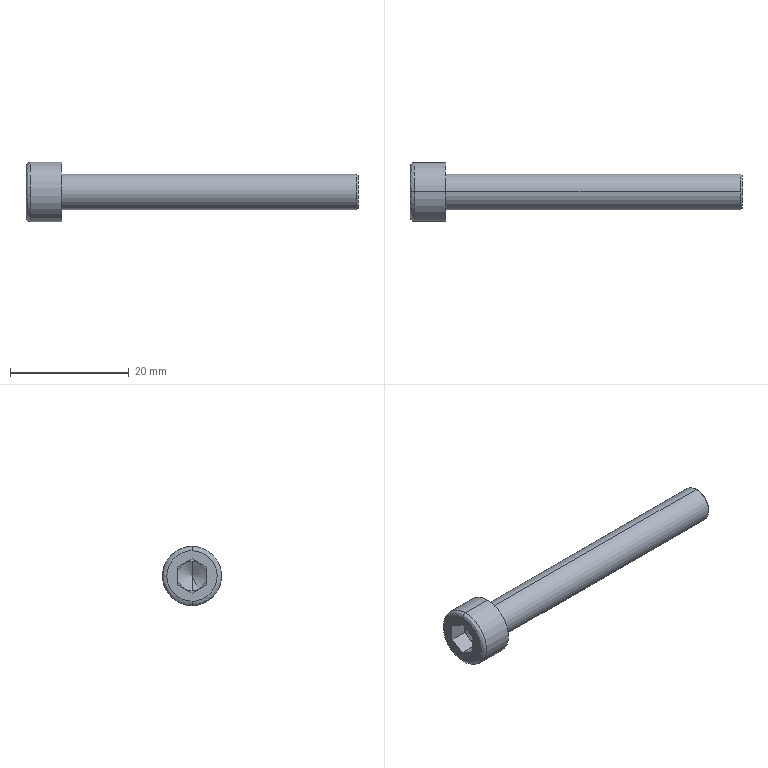Part | STEP file | hexagon socket head cap screws gb_GB_FASTENER_SCREWS_HSHCS M6X50-N | 1 solid | 25 faces | box 56 x 10 x 10 mm | volume 1806 mm3 | plane 15 | cylinder 4 | cone 4 | spline 2 | commonest cylinder face diameters 6 x2 10 x2
STEP:
#1=CARTESIAN_POINT('',(0.75,0.,5.));
#2=VERTEX_POINT('',#1);
#3=CARTESIAN_POINT('',(0.75,0.,-5.));
#4=VERTEX_POINT('',#3);
#5=CARTESIAN_POINT('',(0.75,0.,0.));
#6=DIRECTION('',(1.,0.,0.));
#7=DIRECTION('',(0.,0.,1.));
#8=AXIS2_PLACEMENT_3D('',#5,#6,#7);
#9=CIRCLE('',#8,5.);
#10=EDGE_CURVE('',#2,#4,#9,.T.);
#11=ORIENTED_EDGE('',*,*,#10,.F.);
#12=CARTESIAN_POINT('',(0.,0.,4.25));
#13=VERTEX_POINT('',#12);
#14=CARTESIAN_POINT('',(0.75,0.,4.25));
#15=DIRECTION('',(0.,-1.,0.));
#16=DIRECTION('',(0.,0.,1.));
#17=AXIS2_PLACEMENT_3D('',#14,#15,#16);
#18=CIRCLE('',#17,0.75);
#19=EDGE_CURVE('',#2,#13,#18,.T.);
#20=ORIENTED_EDGE('',*,*,#19,.T.);
#21=CARTESIAN_POINT('',(0.,0.,-4.25));
#22=VERTEX_POINT('',#21);
#23=CARTESIAN_POINT('',(0.,0.,4.25));
#24=CARTESIAN_POINT('',(0.,-8.5,4.25));
#25=CARTESIAN_POINT('',(0.,-8.5,-4.25));
#26=CARTESIAN_POINT('',(0.,0.,-4.25));
#27=(BOUNDED_CURVE()B_SPLINE_CURVE(3,(#23,#24,#25,#26),.UNSPECIFIED.,.F.,.F.)B_SPLINE_CURVE_WITH_KNOTS((4,4),(0.,1.),.UNSPECIFIED.)CURVE()GEOMETRIC_REPRESENTATION_ITEM()RATIONAL_B_SPLINE_CURVE((1.,0.3333,0.3333,1.))REPRESENTATION_ITEM(''));
#28=EDGE_CURVE('',#13,#22,#27,.T.);
#29=ORIENTED_EDGE('',*,*,#28,.T.);
#30=CARTESIAN_POINT('',(0.75,0.,-4.25));
#31=DIRECTION('',(0.,1.,0.));
#32=DIRECTION('',(0.,0.,-1.));
#33=AXIS2_PLACEMENT_3D('',#30,#31,#32);
#34=CIRCLE('',#33,0.75);
#35=EDGE_CURVE('',#4,#22,#34,.T.);
#36=ORIENTED_EDGE('',*,*,#35,.F.);
#37=EDGE_LOOP('',(#11,#20,#29,#36));
#38=FACE_OUTER_BOUND('',#37,.T.);
#39=CARTESIAN_POINT('',(0.75,0.,5.));
#40=CARTESIAN_POINT('',(0.75,-10.,5.));
#41=CARTESIAN_POINT('',(0.75,-10.,-5.));
#42=CARTESIAN_POINT('',(0.75,0.,-5.));
#43=CARTESIAN_POINT('',(0.3107,0.,5.));
#44=CARTESIAN_POINT('',(0.3107,-10.,5.));
#45=CARTESIAN_POINT('',(0.3107,-10.,-5.));
#46=CARTESIAN_POINT('',(0.3107,0.,-5.));
#47=CARTESIAN_POINT('',(0.,0.,4.689));
#48=CARTESIAN_POINT('',(0.,-9.379,4.689));
#49=CARTESIAN_POINT('',(0.,-9.379,-4.689));
#50=CARTESIAN_POINT('',(0.,0.,-4.689));
#51=CARTESIAN_POINT('',(0.,0.,4.25));
#52=CARTESIAN_POINT('',(0.,-8.5,4.25));
#53=CARTESIAN_POINT('',(0.,-8.5,-4.25));
#54=CARTESIAN_POINT('',(0.,0.,-4.25));
#55=(BOUNDED_SURFACE()B_SPLINE_SURFACE(3,3,((#39,#40,#41,#42),(#43,#44,#45,#46),(#47,#48,#49,#50),(#51,#52,#53,#54)),.UNSPECIFIED.,.F.,.F.,.F.)B_SPLINE_SURFACE_WITH_KNOTS((4,4),(4,4),(0.,1.),(0.,1.),.UNSPECIFIED.)GEOMETRIC_REPRESENTATION_ITEM()RATIONAL_B_SPLINE_SURFACE(((1.,0.3333,0.3333,1.),(0.8047,0.2682,0.2682,0.8047),(0.8047,0.2682,0.2682,0.8047),(1.,0.3333,0.3333,1.)))REPRESENTATION_ITEM('')SURFACE());
#56=ADVANCED_FACE('',(#38),#55,.T.);
#57=CARTESIAN_POINT('',(55.75,0.,3.));
#58=VERTEX_POINT('',#57);
#59=CARTESIAN_POINT('',(55.75,0.,-3.));
#60=VERTEX_POINT('',#59);
#61=CARTESIAN_POINT('',(55.75,0.,0.));
#62=DIRECTION('',(-1.,0.,0.));
#63=DIRECTION('',(0.,0.,1.));
#64=AXIS2_PLACEMENT_3D('',#61,#62,#63);
#65=CIRCLE('',#64,3.);
#66=EDGE_CURVE('',#58,#60,#65,.T.);
#67=ORIENTED_EDGE('',*,*,#66,.T.);
#68=CARTESIAN_POINT('',(6.,0.,-3.));
#69=VERTEX_POINT('',#68);
#70=CARTESIAN_POINT('',(56.,0.,-3.));
#71=DIRECTION('',(-1.,0.,0.));
#72=VECTOR('',#71,1000.);
#73=LINE('',#70,#72);
#74=EDGE_CURVE('',#60,#69,#73,.T.);
#75=ORIENTED_EDGE('',*,*,#74,.T.);
#76=CARTESIAN_POINT('',(6.,0.,3.));
#77=VERTEX_POINT('',#76);
#78=CARTESIAN_POINT('',(6.,0.,0.));
#79=DIRECTION('',(1.,0.,0.));
#80=DIRECTION('',(0.,0.,1.));
#81=AXIS2_PLACEMENT_3D('',#78,#79,#80);
#82=CIRCLE('',#81,3.);
#83=EDGE_CURVE('',#69,#77,#82,.T.);
#84=ORIENTED_EDGE('',*,*,#83,.T.);
#85=CARTESIAN_POINT('',(56.,0.,3.));
#86=DIRECTION('',(-1.,0.,0.));
#87=VECTOR('',#86,1000.);
#88=LINE('',#85,#87);
#89=EDGE_CURVE('',#58,#77,#88,.T.);
#90=ORIENTED_EDGE('',*,*,#89,.F.);
#91=EDGE_LOOP('',(#67,#75,#84,#90));
#92=FACE_OUTER_BOUND('',#91,.T.);
#93=CARTESIAN_POINT('',(56.,0.,0.));
#94=DIRECTION('',(-1.,0.,0.));
#95=DIRECTION('',(0.,0.,1.));
#96=AXIS2_PLACEMENT_3D('',#93,#94,#95);
#97=CYLINDRICAL_SURFACE('',#96,3.);
#98=ADVANCED_FACE('',(#92),#97,.T.);
#99=CARTESIAN_POINT('',(56.,0.,2.75));
#100=VERTEX_POINT('',#99);
#101=CARTESIAN_POINT('',(56.,0.,-2.75));
#102=VERTEX_POINT('',#101);
#103=CARTESIAN_POINT('',(56.,0.,0.));
#104=DIRECTION('',(-1.,0.,0.));
#105=DIRECTION('',(0.,0.,1.));
#106=AXIS2_PLACEMENT_3D('',#103,#104,#105);
#107=CIRCLE('',#106,2.75);
#108=EDGE_CURVE('',#100,#102,#107,.T.);
#109=ORIENTED_EDGE('',*,*,#108,.T.);
#110=CARTESIAN_POINT('',(55.75,0.,-3.));
#111=DIRECTION('',(-0.7071,0.,-0.7071));
#112=VECTOR('',#111,1000.);
#113=LINE('',#110,#112);
#114=EDGE_CURVE('',#102,#60,#113,.T.);
#115=ORIENTED_EDGE('',*,*,#114,.T.);
#116=ORIENTED_EDGE('',*,*,#66,.F.);
#117=CARTESIAN_POINT('',(55.75,0.,3.));
#118=DIRECTION('',(-0.7071,0.,0.7071));
#119=VECTOR('',#118,1000.);
#120=LINE('',#117,#119);
#121=EDGE_CURVE('',#100,#58,#120,.T.);
#122=ORIENTED_EDGE('',*,*,#121,.F.);
#123=EDGE_LOOP('',(#109,#115,#116,#122));
#124=FACE_OUTER_BOUND('',#123,.T.);
#125=CARTESIAN_POINT('',(55.75,0.,0.));
#126=DIRECTION('',(-1.,0.,0.));
#127=DIRECTION('',(0.,0.,1.));
#128=AXIS2_PLACEMENT_3D('',#125,#126,#127);
#129=CONICAL_SURFACE('',#128,3.,0.7854);
#130=ADVANCED_FACE('',(#124),#129,.T.);
#131=CARTESIAN_POINT('',(6.,0.,-5.));
#132=VERTEX_POINT('',#131);
#133=CARTESIAN_POINT('',(6.,0.,5.));
#134=VERTEX_POINT('',#133);
#135=CARTESIAN_POINT('',(6.,0.,0.));
#136=DIRECTION('',(1.,0.,0.));
#137=DIRECTION('',(0.,0.,1.));
#138=AXIS2_PLACEMENT_3D('',#135,#136,#137);
#139=CIRCLE('',#138,5.);
#140=EDGE_CURVE('',#132,#134,#139,.T.);
#141=ORIENTED_EDGE('',*,*,#140,.F.);
#142=CARTESIAN_POINT('',(6.,0.,-5.));
#143=DIRECTION('',(-1.,0.,0.));
#144=VECTOR('',#143,1000.);
#145=LINE('',#142,#144);
#146=EDGE_CURVE('',#132,#4,#145,.T.);
#147=ORIENTED_EDGE('',*,*,#146,.T.);
#148=CARTESIAN_POINT('',(0.75,0.,0.));
#149=DIRECTION('',(1.,0.,0.));
#150=DIRECTION('',(0.,0.,1.));
#151=AXIS2_PLACEMENT_3D('',#148,#149,#150);
#152=CIRCLE('',#151,5.);
#153=EDGE_CURVE('',#4,#2,#152,.T.);
#154=ORIENTED_EDGE('',*,*,#153,.T.);
#155=CARTESIAN_POINT('',(6.,0.,5.));
#156=DIRECTION('',(-1.,0.,0.));
#157=VECTOR('',#156,1000.);
#158=LINE('',#155,#157);
#159=EDGE_CURVE('',#134,#2,#158,.T.);
#160=ORIENTED_EDGE('',*,*,#159,.F.);
#161=EDGE_LOOP('',(#141,#147,#154,#160));
#162=FACE_OUTER_BOUND('',#161,.T.);
#163=CARTESIAN_POINT('',(6.,0.,0.));
#164=DIRECTION('',(-1.,0.,0.));
#165=DIRECTION('',(0.,0.,1.));
#166=AXIS2_PLACEMENT_3D('',#163,#164,#165);
#167=CYLINDRICAL_SURFACE('',#166,5.);
#168=ADVANCED_FACE('',(#162),#167,.T.);
#169=CARTESIAN_POINT('',(4.443,0.,0.));
#170=VERTEX_POINT('',#169);
#171=CARTESIAN_POINT('',(3.,0.,2.5));
#172=VERTEX_POINT('',#171);
#173=CARTESIAN_POINT('',(3.,0.,2.5));
#174=DIRECTION('',(-0.5,0.,0.866));
#175=VECTOR('',#174,1000.);
#176=LINE('',#173,#175);
#177=EDGE_CURVE('',#170,#172,#176,.T.);
#178=ORIENTED_EDGE('',*,*,#177,.F.);
#179=CARTESIAN_POINT('',(3.,0.,-2.5));
#180=VERTEX_POINT('',#179);
#181=CARTESIAN_POINT('',(3.,0.,-2.5));
#182=DIRECTION('',(-0.5,0.,-0.866));
#183=VECTOR('',#182,1000.);
#184=LINE('',#181,#183);
#185=EDGE_CURVE('',#170,#180,#184,.T.);
#186=ORIENTED_EDGE('',*,*,#185,.T.);
#187=CARTESIAN_POINT('',(3.,-1.25,-2.165));
#188=VERTEX_POINT('',#187);
#189=CARTESIAN_POINT('',(3.,0.,0.));
#190=DIRECTION('',(1.,0.,0.));
#191=DIRECTION('',(0.,0.,1.));
#192=AXIS2_PLACEMENT_3D('',#189,#190,#191);
#193=CIRCLE('',#192,2.5);
#194=EDGE_CURVE('',#188,#180,#193,.T.);
#195=ORIENTED_EDGE('',*,*,#194,.F.);
#196=CARTESIAN_POINT('',(3.,-2.5,0.));
#197=VERTEX_POINT('',#196);
#198=CARTESIAN_POINT('',(3.,0.,0.));
#199=DIRECTION('',(1.,0.,0.));
#200=DIRECTION('',(0.,0.,1.));
#201=AXIS2_PLACEMENT_3D('',#198,#199,#200);
#202=CIRCLE('',#201,2.5);
#203=EDGE_CURVE('',#197,#188,#202,.T.);
#204=ORIENTED_EDGE('',*,*,#203,.F.);
#205=CARTESIAN_POINT('',(3.,-1.25,2.165));
#206=VERTEX_POINT('',#205);
#207=CARTESIAN_POINT('',(3.,0.,0.));
#208=DIRECTION('',(-1.,0.,0.));
#209=DIRECTION('',(0.,0.,1.));
#210=AXIS2_PLACEMENT_3D('',#207,#208,#209);
#211=CIRCLE('',#210,2.5);
#212=EDGE_CURVE('',#197,#206,#211,.T.);
#213=ORIENTED_EDGE('',*,*,#212,.T.);
#214=CARTESIAN_POINT('',(3.,0.,0.));
#215=DIRECTION('',(1.,0.,0.));
#216=DIRECTION('',(0.,0.,1.));
#217=AXIS2_PLACEMENT_3D('',#214,#215,#216);
#218=CIRCLE('',#217,2.5);
#219=EDGE_CURVE('',#172,#206,#218,.T.);
#220=ORIENTED_EDGE('',*,*,#219,.F.);
#221=EDGE_LOOP('',(#178,#186,#195,#204,#213,#220));
#222=FACE_OUTER_BOUND('',#221,.T.);
#223=CARTESIAN_POINT('',(3.,0.,0.));
#224=DIRECTION('',(-1.,0.,0.));
#225=DIRECTION('',(0.,0.,1.));
#226=AXIS2_PLACEMENT_3D('',#223,#224,#225);
#227=CONICAL_SURFACE('',#226,2.5,1.047);
#228=ADVANCED_FACE('',(#222),#227,.F.);
#229=ORIENTED_EDGE('',*,*,#74,.F.);
#230=CARTESIAN_POINT('',(55.75,0.,0.));
#231=DIRECTION('',(-1.,0.,0.));
#232=DIRECTION('',(0.,0.,1.));
#233=AXIS2_PLACEMENT_3D('',#230,#231,#232);
#234=CIRCLE('',#233,3.);
#235=EDGE_CURVE('',#60,#58,#234,.T.);
#236=ORIENTED_EDGE('',*,*,#235,.T.);
#237=ORIENTED_EDGE('',*,*,#89,.T.);
#238=CARTESIAN_POINT('',(6.,0.,0.));
#239=DIRECTION('',(1.,0.,0.));
#240=DIRECTION('',(0.,0.,1.));
#241=AXIS2_PLACEMENT_3D('',#238,#239,#240);
#242=CIRCLE('',#241,3.);
#243=EDGE_CURVE('',#77,#69,#242,.T.);
#244=ORIENTED_EDGE('',*,*,#243,.T.);
#245=EDGE_LOOP('',(#229,#236,#237,#244));
#246=FACE_OUTER_BOUND('',#245,.T.);
#247=CARTESIAN_POINT('',(56.,0.,0.));
#248=DIRECTION('',(-1.,0.,0.));
#249=DIRECTION('',(0.,0.,1.));
#250=AXIS2_PLACEMENT_3D('',#247,#248,#249);
#251=CYLINDRICAL_SURFACE('',#250,3.);
#252=ADVANCED_FACE('',(#246),#251,.T.);
#253=ORIENTED_EDGE('',*,*,#243,.F.);
#254=ORIENTED_EDGE('',*,*,#83,.F.);
#255=EDGE_LOOP('',(#253,#254));
#256=FACE_BOUND('',#255,.T.);
#257=CARTESIAN_POINT('',(6.,0.,0.));
#258=DIRECTION('',(1.,0.,0.));
#259=DIRECTION('',(0.,0.,1.));
#260=AXIS2_PLACEMENT_3D('',#257,#258,#259);
#261=CIRCLE('',#260,5.);
#262=EDGE_CURVE('',#134,#132,#261,.T.);
#263=ORIENTED_EDGE('',*,*,#262,.T.);
#264=ORIENTED_EDGE('',*,*,#140,.T.);
#265=EDGE_LOOP('',(#263,#264));
#266=FACE_OUTER_BOUND('',#265,.T.);
#267=CARTESIAN_POINT('',(6.,0.,0.));
#268=DIRECTION('',(1.,0.,0.));
#269=DIRECTION('',(0.,0.,-1.));
#270=AXIS2_PLACEMENT_3D('',#267,#268,#269);
#271=PLANE('',#270);
#272=ADVANCED_FACE('',(#256,#266),#271,.T.);
#273=ORIENTED_EDGE('',*,*,#114,.F.);
#274=CARTESIAN_POINT('',(56.,0.,0.));
#275=DIRECTION('',(-1.,0.,0.));
#276=DIRECTION('',(0.,0.,1.));
#277=AXIS2_PLACEMENT_3D('',#274,#275,#276);
#278=CIRCLE('',#277,2.75);
#279=EDGE_CURVE('',#102,#100,#278,.T.);
#280=ORIENTED_EDGE('',*,*,#279,.T.);
#281=ORIENTED_EDGE('',*,*,#121,.T.);
#282=ORIENTED_EDGE('',*,*,#235,.F.);
#283=EDGE_LOOP('',(#273,#280,#281,#282));
#284=FACE_OUTER_BOUND('',#283,.T.);
#285=CARTESIAN_POINT('',(55.75,0.,0.));
#286=DIRECTION('',(-1.,0.,0.));
#287=DIRECTION('',(0.,0.,1.));
#288=AXIS2_PLACEMENT_3D('',#285,#286,#287);
#289=CONICAL_SURFACE('',#288,3.,0.7854);
#290=ADVANCED_FACE('',(#284),#289,.T.);
#291=ORIENTED_EDGE('',*,*,#146,.F.);
#292=ORIENTED_EDGE('',*,*,#262,.F.);
#293=ORIENTED_EDGE('',*,*,#159,.T.);
#294=ORIENTED_EDGE('',*,*,#10,.T.);
#295=EDGE_LOOP('',(#291,#292,#293,#294));
#296=FACE_OUTER_BOUND('',#295,.T.);
#297=CARTESIAN_POINT('',(6.,0.,0.));
#298=DIRECTION('',(-1.,0.,0.));
#299=DIRECTION('',(0.,0.,1.));
#300=AXIS2_PLACEMENT_3D('',#297,#298,#299);
#301=CYLINDRICAL_SURFACE('',#300,5.);
#302=ADVANCED_FACE('',(#296),#301,.T.);
#303=ORIENTED_EDGE('',*,*,#108,.F.);
#304=ORIENTED_EDGE('',*,*,#279,.F.);
#305=EDGE_LOOP('',(#303,#304));
#306=FACE_OUTER_BOUND('',#305,.T.);
#307=CARTESIAN_POINT('',(56.,0.,0.));
#308=DIRECTION('',(1.,0.,0.));
#309=DIRECTION('',(0.,0.,-1.));
#310=AXIS2_PLACEMENT_3D('',#307,#308,#309);
#311=PLANE('',#310);
#312=ADVANCED_FACE('',(#306),#311,.T.);
#313=ORIENTED_EDGE('',*,*,#19,.F.);
#314=ORIENTED_EDGE('',*,*,#153,.F.);
#315=ORIENTED_EDGE('',*,*,#35,.T.);
#316=CARTESIAN_POINT('',(0.,0.,-4.25));
#317=CARTESIAN_POINT('',(0.,8.5,-4.25));
#318=CARTESIAN_POINT('',(0.,8.5,4.25));
#319=CARTESIAN_POINT('',(0.,0.,4.25));
#320=(BOUNDED_CURVE()B_SPLINE_CURVE(3,(#316,#317,#318,#319),.UNSPECIFIED.,.F.,.F.)B_SPLINE_CURVE_WITH_KNOTS((4,4),(0.,1.),.UNSPECIFIED.)CURVE()GEOMETRIC_REPRESENTATION_ITEM()RATIONAL_B_SPLINE_CURVE((1.,0.3333,0.3333,1.))REPRESENTATION_ITEM(''));
#321=EDGE_CURVE('',#22,#13,#320,.T.);
#322=ORIENTED_EDGE('',*,*,#321,.T.);
#323=EDGE_LOOP('',(#313,#314,#315,#322));
#324=FACE_OUTER_BOUND('',#323,.T.);
#325=CARTESIAN_POINT('',(0.75,0.,-5.));
#326=CARTESIAN_POINT('',(0.75,10.,-5.));
#327=CARTESIAN_POINT('',(0.75,10.,5.));
#328=CARTESIAN_POINT('',(0.75,0.,5.));
#329=CARTESIAN_POINT('',(0.3107,0.,-5.));
#330=CARTESIAN_POINT('',(0.3107,10.,-5.));
#331=CARTESIAN_POINT('',(0.3107,10.,5.));
#332=CARTESIAN_POINT('',(0.3107,0.,5.));
#333=CARTESIAN_POINT('',(0.,0.,-4.689));
#334=CARTESIAN_POINT('',(0.,9.379,-4.689));
#335=CARTESIAN_POINT('',(0.,9.379,4.689));
#336=CARTESIAN_POINT('',(0.,0.,4.689));
#337=CARTESIAN_POINT('',(0.,0.,-4.25));
#338=CARTESIAN_POINT('',(0.,8.5,-4.25));
#339=CARTESIAN_POINT('',(0.,8.5,4.25));
#340=CARTESIAN_POINT('',(0.,0.,4.25));
#341=(BOUNDED_SURFACE()B_SPLINE_SURFACE(3,3,((#325,#326,#327,#328),(#329,#330,#331,#332),(#333,#334,#335,#336),(#337,#338,#339,#340)),.UNSPECIFIED.,.F.,.F.,.F.)B_SPLINE_SURFACE_WITH_KNOTS((4,4),(4,4),(0.,1.),(0.,1.),.UNSPECIFIED.)GEOMETRIC_REPRESENTATION_ITEM()RATIONAL_B_SPLINE_SURFACE(((1.,0.3333,0.3333,1.),(0.8047,0.2682,0.2682,0.8047),(0.8047,0.2682,0.2682,0.8047),(1.,0.3333,0.3333,1.)))REPRESENTATION_ITEM('')SURFACE());
#342=ADVANCED_FACE('',(#324),#341,.T.);
#343=CARTESIAN_POINT('',(0.,2.5,-1.443));
#344=VERTEX_POINT('',#343);
#345=CARTESIAN_POINT('',(0.,0.,-2.887));
#346=VERTEX_POINT('',#345);
#347=CARTESIAN_POINT('',(0.,2.5,-1.443));
#348=DIRECTION('',(0.,-0.866,-0.5));
#349=VECTOR('',#348,1000.);
#350=LINE('',#347,#349);
#351=EDGE_CURVE('',#344,#346,#350,.T.);
#352=ORIENTED_EDGE('',*,*,#351,.F.);
#353=CARTESIAN_POINT('',(0.,2.5,1.443));
#354=VERTEX_POINT('',#353);
#355=CARTESIAN_POINT('',(0.,2.5,0.));
#356=DIRECTION('',(0.,0.,-1.));
#357=VECTOR('',#356,1000.);
#358=LINE('',#355,#357);
#359=EDGE_CURVE('',#354,#344,#358,.T.);
#360=ORIENTED_EDGE('',*,*,#359,.F.);
#361=CARTESIAN_POINT('',(0.,0.,2.887));
#362=VERTEX_POINT('',#361);
#363=CARTESIAN_POINT('',(0.,0.,2.887));
#364=DIRECTION('',(0.,0.866,-0.5));
#365=VECTOR('',#364,1000.);
#366=LINE('',#363,#365);
#367=EDGE_CURVE('',#362,#354,#366,.T.);
#368=ORIENTED_EDGE('',*,*,#367,.F.);
#369=CARTESIAN_POINT('',(0.,-2.5,1.443));
#370=VERTEX_POINT('',#369);
#371=CARTESIAN_POINT('',(0.,-2.5,1.443));
#372=DIRECTION('',(0.,0.866,0.5));
#373=VECTOR('',#372,1000.);
#374=LINE('',#371,#373);
#375=EDGE_CURVE('',#370,#362,#374,.T.);
#376=ORIENTED_EDGE('',*,*,#375,.F.);
#377=CARTESIAN_POINT('',(0.,-2.5,-1.443));
#378=VERTEX_POINT('',#377);
#379=CARTESIAN_POINT('',(0.,-2.5,0.));
#380=DIRECTION('',(0.,0.,1.));
#381=VECTOR('',#380,1000.);
#382=LINE('',#379,#381);
#383=EDGE_CURVE('',#378,#370,#382,.T.);
#384=ORIENTED_EDGE('',*,*,#383,.F.);
#385=CARTESIAN_POINT('',(0.,0.,-2.887));
#386=DIRECTION('',(0.,-0.866,0.5));
#387=VECTOR('',#386,1000.);
#388=LINE('',#385,#387);
#389=EDGE_CURVE('',#346,#378,#388,.T.);
#390=ORIENTED_EDGE('',*,*,#389,.F.);
#391=EDGE_LOOP('',(#352,#360,#368,#376,#384,#390));
#392=FACE_BOUND('',#391,.T.);
#393=ORIENTED_EDGE('',*,*,#321,.F.);
#394=ORIENTED_EDGE('',*,*,#28,.F.);
#395=EDGE_LOOP('',(#393,#394));
#396=FACE_OUTER_BOUND('',#395,.T.);
#397=CARTESIAN_POINT('',(0.,0.,0.));
#398=DIRECTION('',(1.,0.,0.));
#399=DIRECTION('',(0.,0.,-1.));
#400=AXIS2_PLACEMENT_3D('',#397,#398,#399);
#401=PLANE('',#400);
#402=ADVANCED_FACE('',(#392,#396),#401,.F.);
#403=CARTESIAN_POINT('',(3.,0.,-2.887));
#404=VERTEX_POINT('',#403);
#405=CARTESIAN_POINT('',(3.,-2.5,-1.443));
#406=DIRECTION('',(0.,0.866,-0.5));
#407=VECTOR('',#406,1000.);
#408=LINE('',#405,#407);
#409=EDGE_CURVE('',#188,#404,#408,.T.);
#410=ORIENTED_EDGE('',*,*,#409,.T.);
#411=CARTESIAN_POINT('',(3.,0.,-2.887));
#412=DIRECTION('',(-1.,0.,0.));
#413=VECTOR('',#412,1000.);
#414=LINE('',#411,#413);
#415=EDGE_CURVE('',#404,#346,#414,.T.);
#416=ORIENTED_EDGE('',*,*,#415,.T.);
#417=ORIENTED_EDGE('',*,*,#389,.T.);
#418=CARTESIAN_POINT('',(3.,-2.5,-1.443));
#419=VERTEX_POINT('',#418);
#420=CARTESIAN_POINT('',(3.,-2.5,-1.443));
#421=DIRECTION('',(1.,0.,0.));
#422=VECTOR('',#421,1000.);
#423=LINE('',#420,#422);
#424=EDGE_CURVE('',#378,#419,#423,.T.);
#425=ORIENTED_EDGE('',*,*,#424,.T.);
#426=CARTESIAN_POINT('',(3.,-2.5,-1.443));
#427=DIRECTION('',(0.,0.866,-0.5));
#428=VECTOR('',#427,1000.);
#429=LINE('',#426,#428);
#430=EDGE_CURVE('',#419,#188,#429,.T.);
#431=ORIENTED_EDGE('',*,*,#430,.T.);
#432=EDGE_LOOP('',(#410,#416,#417,#425,#431));
#433=FACE_OUTER_BOUND('',#432,.T.);
#434=CARTESIAN_POINT('',(3.,-2.5,-1.443));
#435=DIRECTION('',(0.,0.5,0.866));
#436=DIRECTION('',(0.,-0.866,0.5));
#437=AXIS2_PLACEMENT_3D('',#434,#435,#436);
#438=PLANE('',#437);
#439=ADVANCED_FACE('',(#433),#438,.T.);
#440=CARTESIAN_POINT('',(3.,1.25,-2.165));
#441=VERTEX_POINT('',#440);
#442=CARTESIAN_POINT('',(3.,2.5,-1.443));
#443=VERTEX_POINT('',#442);
#444=CARTESIAN_POINT('',(3.,1.25,-2.165));
#445=DIRECTION('',(0.,0.866,0.5));
#446=VECTOR('',#445,1000.);
#447=LINE('',#444,#446);
#448=EDGE_CURVE('',#441,#443,#447,.T.);
#449=ORIENTED_EDGE('',*,*,#448,.T.);
#450=CARTESIAN_POINT('',(3.,2.5,-1.443));
#451=DIRECTION('',(-1.,0.,0.));
#452=VECTOR('',#451,1000.);
#453=LINE('',#450,#452);
#454=EDGE_CURVE('',#443,#344,#453,.T.);
#455=ORIENTED_EDGE('',*,*,#454,.T.);
#456=ORIENTED_EDGE('',*,*,#351,.T.);
#457=ORIENTED_EDGE('',*,*,#415,.F.);
#458=CARTESIAN_POINT('',(3.,0.,-2.887));
#459=DIRECTION('',(0.,0.866,0.5));
#460=VECTOR('',#459,1000.);
#461=LINE('',#458,#460);
#462=EDGE_CURVE('',#404,#441,#461,.T.);
#463=ORIENTED_EDGE('',*,*,#462,.T.);
#464=EDGE_LOOP('',(#449,#455,#456,#457,#463));
#465=FACE_OUTER_BOUND('',#464,.T.);
#466=CARTESIAN_POINT('',(3.,0.,-2.887));
#467=DIRECTION('',(0.,-0.5,0.866));
#468=DIRECTION('',(0.,-0.866,-0.5));
#469=AXIS2_PLACEMENT_3D('',#466,#467,#468);
#470=PLANE('',#469);
#471=ADVANCED_FACE('',(#465),#470,.T.);
#472=CARTESIAN_POINT('',(3.,2.5,0.));
#473=VERTEX_POINT('',#472);
#474=CARTESIAN_POINT('',(3.,2.5,1.443));
#475=VERTEX_POINT('',#474);
#476=CARTESIAN_POINT('',(3.,2.5,-2.887));
#477=DIRECTION('',(0.,0.,1.));
#478=VECTOR('',#477,1000.);
#479=LINE('',#476,#478);
#480=EDGE_CURVE('',#473,#475,#479,.T.);
#481=ORIENTED_EDGE('',*,*,#480,.T.);
#482=CARTESIAN_POINT('',(3.,2.5,1.443));
#483=DIRECTION('',(-1.,0.,0.));
#484=VECTOR('',#483,1000.);
#485=LINE('',#482,#484);
#486=EDGE_CURVE('',#475,#354,#485,.T.);
#487=ORIENTED_EDGE('',*,*,#486,.T.);
#488=ORIENTED_EDGE('',*,*,#359,.T.);
#489=ORIENTED_EDGE('',*,*,#454,.F.);
#490=CARTESIAN_POINT('',(3.,2.5,-2.887));
#491=DIRECTION('',(0.,0.,1.));
#492=VECTOR('',#491,1000.);
#493=LINE('',#490,#492);
#494=EDGE_CURVE('',#443,#473,#493,.T.);
#495=ORIENTED_EDGE('',*,*,#494,.T.);
#496=EDGE_LOOP('',(#481,#487,#488,#489,#495));
#497=FACE_OUTER_BOUND('',#496,.T.);
#498=CARTESIAN_POINT('',(3.,2.5,-1.443));
#499=DIRECTION('',(0.,-1.,0.));
#500=DIRECTION('',(0.,0.,-1.));
#501=AXIS2_PLACEMENT_3D('',#498,#499,#500);
#502=PLANE('',#501);
#503=ADVANCED_FACE('',(#497),#502,.T.);
#504=CARTESIAN_POINT('',(3.,1.25,2.165));
#505=VERTEX_POINT('',#504);
#506=CARTESIAN_POINT('',(3.,0.,2.887));
#507=VERTEX_POINT('',#506);
#508=CARTESIAN_POINT('',(3.,2.5,1.443));
#509=DIRECTION('',(0.,-0.866,0.5));
#510=VECTOR('',#509,1000.);
#511=LINE('',#508,#510);
#512=EDGE_CURVE('',#505,#507,#511,.T.);
#513=ORIENTED_EDGE('',*,*,#512,.T.);
#514=CARTESIAN_POINT('',(3.,0.,2.887));
#515=DIRECTION('',(-1.,0.,0.));
#516=VECTOR('',#515,1000.);
#517=LINE('',#514,#516);
#518=EDGE_CURVE('',#507,#362,#517,.T.);
#519=ORIENTED_EDGE('',*,*,#518,.T.);
#520=ORIENTED_EDGE('',*,*,#367,.T.);
#521=ORIENTED_EDGE('',*,*,#486,.F.);
#522=CARTESIAN_POINT('',(3.,2.5,1.443));
#523=DIRECTION('',(0.,-0.866,0.5));
#524=VECTOR('',#523,1000.);
#525=LINE('',#522,#524);
#526=EDGE_CURVE('',#475,#505,#525,.T.);
#527=ORIENTED_EDGE('',*,*,#526,.T.);
#528=EDGE_LOOP('',(#513,#519,#520,#521,#527));
#529=FACE_OUTER_BOUND('',#528,.T.);
#530=CARTESIAN_POINT('',(3.,2.5,1.443));
#531=DIRECTION('',(0.,-0.5,-0.866));
#532=DIRECTION('',(0.,0.866,-0.5));
#533=AXIS2_PLACEMENT_3D('',#530,#531,#532);
#534=PLANE('',#533);
#535=ADVANCED_FACE('',(#529),#534,.T.);
#536=CARTESIAN_POINT('',(3.,-2.5,1.443));
#537=VERTEX_POINT('',#536);
#538=CARTESIAN_POINT('',(3.,0.,2.887));
#539=DIRECTION('',(0.,-0.866,-0.5));
#540=VECTOR('',#539,1000.);
#541=LINE('',#538,#540);
#542=EDGE_CURVE('',#206,#537,#541,.T.);
#543=ORIENTED_EDGE('',*,*,#542,.T.);
#544=CARTESIAN_POINT('',(3.,-2.5,1.443));
#545=DIRECTION('',(-1.,0.,0.));
#546=VECTOR('',#545,1000.);
#547=LINE('',#544,#546);
#548=EDGE_CURVE('',#537,#370,#547,.T.);
#549=ORIENTED_EDGE('',*,*,#548,.T.);
#550=ORIENTED_EDGE('',*,*,#375,.T.);
#551=ORIENTED_EDGE('',*,*,#518,.F.);
#552=CARTESIAN_POINT('',(3.,0.,2.887));
#553=DIRECTION('',(0.,-0.866,-0.5));
#554=VECTOR('',#553,1000.);
#555=LINE('',#552,#554);
#556=EDGE_CURVE('',#507,#206,#555,.T.);
#557=ORIENTED_EDGE('',*,*,#556,.T.);
#558=EDGE_LOOP('',(#543,#549,#550,#551,#557));
#559=FACE_OUTER_BOUND('',#558,.T.);
#560=CARTESIAN_POINT('',(3.,0.,2.887));
#561=DIRECTION('',(0.,0.5,-0.866));
#562=DIRECTION('',(0.,0.866,0.5));
#563=AXIS2_PLACEMENT_3D('',#560,#561,#562);
#564=PLANE('',#563);
#565=ADVANCED_FACE('',(#559),#564,.T.);
#566=CARTESIAN_POINT('',(3.,-2.5,-2.887));
#567=DIRECTION('',(0.,0.,-1.));
#568=VECTOR('',#567,1000.);
#569=LINE('',#566,#568);
#570=EDGE_CURVE('',#197,#419,#569,.T.);
#571=ORIENTED_EDGE('',*,*,#570,.T.);
#572=ORIENTED_EDGE('',*,*,#424,.F.);
#573=ORIENTED_EDGE('',*,*,#383,.T.);
#574=ORIENTED_EDGE('',*,*,#548,.F.);
#575=CARTESIAN_POINT('',(3.,-2.5,1.443));
#576=DIRECTION('',(0.,0.,-1.));
#577=VECTOR('',#576,1000.);
#578=LINE('',#575,#577);
#579=EDGE_CURVE('',#537,#197,#578,.T.);
#580=ORIENTED_EDGE('',*,*,#579,.T.);
#581=EDGE_LOOP('',(#571,#572,#573,#574,#580));
#582=FACE_OUTER_BOUND('',#581,.T.);
#583=CARTESIAN_POINT('',(3.,-2.5,1.443));
#584=DIRECTION('',(0.,1.,0.));
#585=DIRECTION('',(0.,0.,1.));
#586=AXIS2_PLACEMENT_3D('',#583,#584,#585);
#587=PLANE('',#586);
#588=ADVANCED_FACE('',(#582),#587,.T.);
#589=ORIENTED_EDGE('',*,*,#462,.F.);
#590=ORIENTED_EDGE('',*,*,#409,.F.);
#591=ORIENTED_EDGE('',*,*,#194,.T.);
#592=CARTESIAN_POINT('',(3.,0.,0.));
#593=DIRECTION('',(1.,0.,0.));
#594=DIRECTION('',(0.,0.,1.));
#595=AXIS2_PLACEMENT_3D('',#592,#593,#594);
#596=CIRCLE('',#595,2.5);
#597=EDGE_CURVE('',#180,#441,#596,.T.);
#598=ORIENTED_EDGE('',*,*,#597,.T.);
#599=EDGE_LOOP('',(#589,#590,#591,#598));
#600=FACE_OUTER_BOUND('',#599,.T.);
#601=CARTESIAN_POINT('',(3.,0.,-2.887));
#602=DIRECTION('',(1.,0.,0.));
#603=DIRECTION('',(0.,0.,-1.));
#604=AXIS2_PLACEMENT_3D('',#601,#602,#603);
#605=PLANE('',#604);
#606=ADVANCED_FACE('',(#600),#605,.F.);
#607=ORIENTED_EDGE('',*,*,#556,.F.);
#608=ORIENTED_EDGE('',*,*,#512,.F.);
#609=CARTESIAN_POINT('',(3.,0.,0.));
#610=DIRECTION('',(1.,0.,0.));
#611=DIRECTION('',(0.,0.,1.));
#612=AXIS2_PLACEMENT_3D('',#609,#610,#611);
#613=CIRCLE('',#612,2.5);
#614=EDGE_CURVE('',#505,#172,#613,.T.);
#615=ORIENTED_EDGE('',*,*,#614,.T.);
#616=ORIENTED_EDGE('',*,*,#219,.T.);
#617=EDGE_LOOP('',(#607,#608,#615,#616));
#618=FACE_OUTER_BOUND('',#617,.T.);
#619=CARTESIAN_POINT('',(3.,0.,-2.887));
#620=DIRECTION('',(1.,0.,0.));
#621=DIRECTION('',(0.,0.,-1.));
#622=AXIS2_PLACEMENT_3D('',#619,#620,#621);
#623=PLANE('',#622);
#624=ADVANCED_FACE('',(#618),#623,.F.);
#625=ORIENTED_EDGE('',*,*,#579,.F.);
#626=ORIENTED_EDGE('',*,*,#542,.F.);
#627=ORIENTED_EDGE('',*,*,#212,.F.);
#628=EDGE_LOOP('',(#625,#626,#627));
#629=FACE_OUTER_BOUND('',#628,.T.);
#630=CARTESIAN_POINT('',(3.,0.,-2.887));
#631=DIRECTION('',(1.,0.,0.));
#632=DIRECTION('',(0.,0.,-1.));
#633=AXIS2_PLACEMENT_3D('',#630,#631,#632);
#634=PLANE('',#633);
#635=ADVANCED_FACE('',(#629),#634,.F.);
#636=ORIENTED_EDGE('',*,*,#185,.F.);
#637=ORIENTED_EDGE('',*,*,#177,.T.);
#638=ORIENTED_EDGE('',*,*,#614,.F.);
#639=CARTESIAN_POINT('',(3.,0.,0.));
#640=DIRECTION('',(1.,0.,0.));
#641=DIRECTION('',(0.,0.,1.));
#642=AXIS2_PLACEMENT_3D('',#639,#640,#641);
#643=CIRCLE('',#642,2.5);
#644=EDGE_CURVE('',#473,#505,#643,.T.);
#645=ORIENTED_EDGE('',*,*,#644,.F.);
#646=CARTESIAN_POINT('',(3.,0.,0.));
#647=DIRECTION('',(1.,0.,0.));
#648=DIRECTION('',(0.,0.,1.));
#649=AXIS2_PLACEMENT_3D('',#646,#647,#648);
#650=CIRCLE('',#649,2.5);
#651=EDGE_CURVE('',#441,#473,#650,.T.);
#652=ORIENTED_EDGE('',*,*,#651,.F.);
#653=ORIENTED_EDGE('',*,*,#597,.F.);
#654=EDGE_LOOP('',(#636,#637,#638,#645,#652,#653));
#655=FACE_OUTER_BOUND('',#654,.T.);
#656=CARTESIAN_POINT('',(3.,0.,0.));
#657=DIRECTION('',(-1.,0.,0.));
#658=DIRECTION('',(0.,0.,1.));
#659=AXIS2_PLACEMENT_3D('',#656,#657,#658);
#660=CONICAL_SURFACE('',#659,2.5,1.047);
#661=ADVANCED_FACE('',(#655),#660,.F.);
#662=ORIENTED_EDGE('',*,*,#430,.F.);
#663=ORIENTED_EDGE('',*,*,#570,.F.);
#664=ORIENTED_EDGE('',*,*,#203,.T.);
#665=EDGE_LOOP('',(#662,#663,#664));
#666=FACE_OUTER_BOUND('',#665,.T.);
#667=CARTESIAN_POINT('',(3.,0.,-2.887));
#668=DIRECTION('',(1.,0.,0.));
#669=DIRECTION('',(0.,0.,-1.));
#670=AXIS2_PLACEMENT_3D('',#667,#668,#669);
#671=PLANE('',#670);
#672=ADVANCED_FACE('',(#666),#671,.F.);
#673=ORIENTED_EDGE('',*,*,#526,.F.);
#674=ORIENTED_EDGE('',*,*,#480,.F.);
#675=ORIENTED_EDGE('',*,*,#644,.T.);
#676=EDGE_LOOP('',(#673,#674,#675));
#677=FACE_OUTER_BOUND('',#676,.T.);
#678=CARTESIAN_POINT('',(3.,0.,-2.887));
#679=DIRECTION('',(1.,0.,0.));
#680=DIRECTION('',(0.,0.,-1.));
#681=AXIS2_PLACEMENT_3D('',#678,#679,#680);
#682=PLANE('',#681);
#683=ADVANCED_FACE('',(#677),#682,.F.);
#684=ORIENTED_EDGE('',*,*,#494,.F.);
#685=ORIENTED_EDGE('',*,*,#448,.F.);
#686=ORIENTED_EDGE('',*,*,#651,.T.);
#687=EDGE_LOOP('',(#684,#685,#686));
#688=FACE_OUTER_BOUND('',#687,.T.);
#689=CARTESIAN_POINT('',(3.,0.,-2.887));
#690=DIRECTION('',(1.,0.,0.));
#691=DIRECTION('',(0.,0.,-1.));
#692=AXIS2_PLACEMENT_3D('',#689,#690,#691);
#693=PLANE('',#692);
#694=ADVANCED_FACE('',(#688),#693,.F.);
#695=CLOSED_SHELL('',(#56,#98,#130,#168,#228,#252,#272,#290,#302,#312,#342,#402,#439,#471,#503,#535,#565,#588,#606,#624,#635,#661,#672,#683,#694));
#696=MANIFOLD_SOLID_BREP('',#695);
#697=CARTESIAN_POINT('',(0.,0.,0.));
#698=DIRECTION('',(0.,0.,1.));
#699=DIRECTION('',(1.,0.,0.));
#700=AXIS2_PLACEMENT_3D('',#697,#698,#699);
#701=(LENGTH_UNIT()NAMED_UNIT(*)SI_UNIT(.MILLI.,.METRE.));
#702=UNCERTAINTY_MEASURE_WITH_UNIT(LENGTH_MEASURE(0.00001),#701,'','');
#703=(NAMED_UNIT(*)PLANE_ANGLE_UNIT()SI_UNIT($,.RADIAN.));
#704=(NAMED_UNIT(*)SI_UNIT($,.STERADIAN.)SOLID_ANGLE_UNIT());
#705=(GEOMETRIC_REPRESENTATION_CONTEXT(3)GLOBAL_UNCERTAINTY_ASSIGNED_CONTEXT((#702))GLOBAL_UNIT_ASSIGNED_CONTEXT((#701,#703,#704))REPRESENTATION_CONTEXT('',''));
#706=ADVANCED_BREP_SHAPE_REPRESENTATION('',(#696,#700),#705);